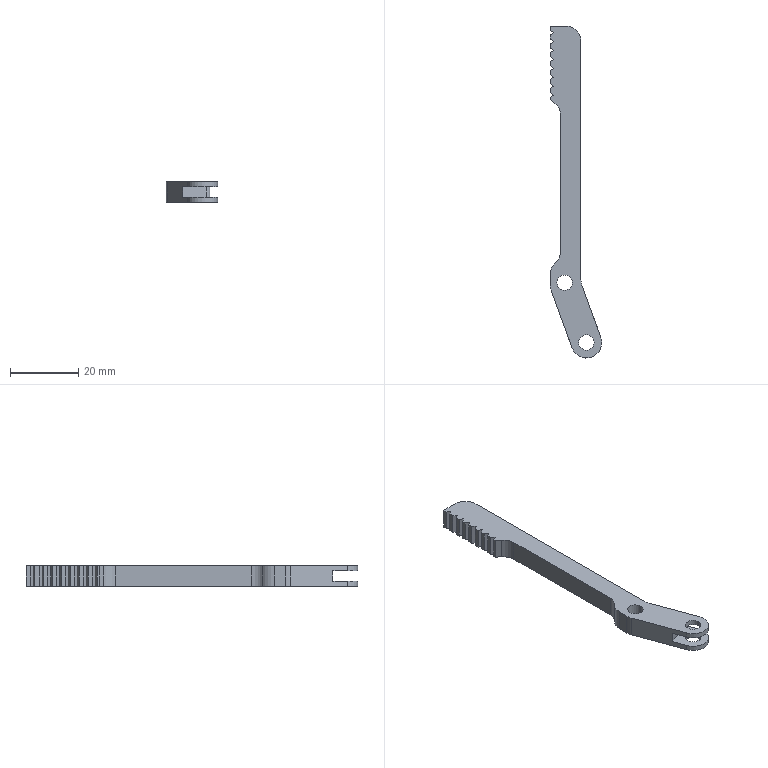Part | SolidWorks | features HoleWzd 3, ICE 3, Fillet 2, Extrusion 1, Scale 1 | 1 solid | 54 faces | box 15.09 x 97.026 x 6 mm | volume 3984 mm3 | plane 37 | cylinder 17 | commonest cylinder face diameters 9 x10 4.5 x6 3 x1